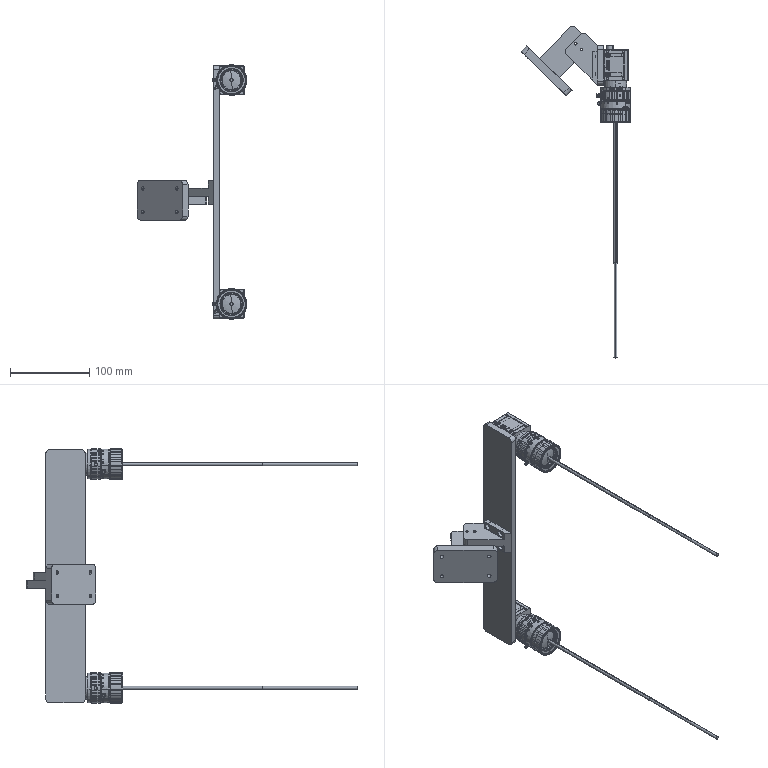Part | SolidWorks | features LocalLPattern 1, ReferencePattern 1 | 43 solids | 11849 faces | volume 394201 mm3 | plane 8441 | cylinder 2260 | spline 548 | cone 528 | torus 72 | commonest cylinder face diameters 1.6 x370 4 x154 2 x150 37.5 x114 1.201 x98 38.6 x86